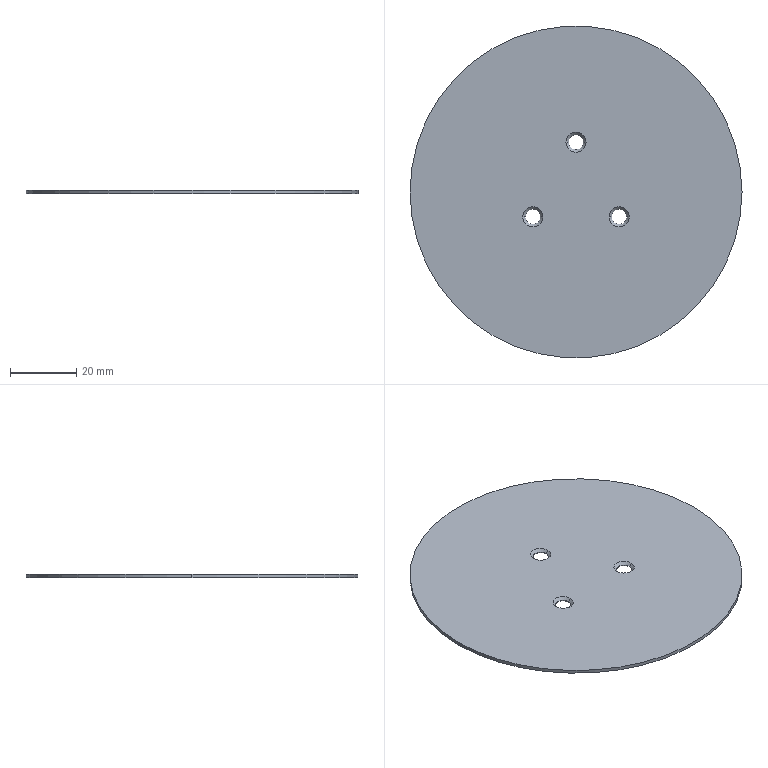Part | SolidWorks | features Chamfer 1, Extrusion 1 | 1 solid | 16 faces | box 100 x 100 x 1 mm | volume 7791 mm3 | cylinder 8 | cone 6 | plane 2 | commonest cylinder face diameters 4.5 x6 100 x2
STEP:
#1=CARTESIAN_POINT('',(-2.25,15.,0.2));
#2=VERTEX_POINT('',#1);
#3=CARTESIAN_POINT('',(2.25,15.,0.2));
#4=VERTEX_POINT('',#3);
#5=CARTESIAN_POINT('',(0.,15.,0.2));
#6=DIRECTION('',(0.,0.,1.));
#7=DIRECTION('',(1.,0.,0.));
#8=AXIS2_PLACEMENT_3D('',#5,#6,#7);
#9=CIRCLE('',#8,2.25);
#10=EDGE_CURVE('',#2,#4,#9,.T.);
#11=ORIENTED_EDGE('',*,*,#10,.F.);
#12=CARTESIAN_POINT('',(-3.05,15.,1.));
#13=VERTEX_POINT('',#12);
#14=CARTESIAN_POINT('',(-2.25,15.,0.2));
#15=DIRECTION('',(-0.7071,0.,0.7071));
#16=VECTOR('',#15,1000.);
#17=LINE('',#14,#16);
#18=EDGE_CURVE('',#2,#13,#17,.T.);
#19=ORIENTED_EDGE('',*,*,#18,.T.);
#20=CARTESIAN_POINT('',(3.05,15.,1.));
#21=VERTEX_POINT('',#20);
#22=CARTESIAN_POINT('',(0.,15.,1.));
#23=DIRECTION('',(0.,0.,-1.));
#24=DIRECTION('',(1.,0.,0.));
#25=AXIS2_PLACEMENT_3D('',#22,#23,#24);
#26=CIRCLE('',#25,3.05);
#27=EDGE_CURVE('',#21,#13,#26,.T.);
#28=ORIENTED_EDGE('',*,*,#27,.F.);
#29=CARTESIAN_POINT('',(2.25,15.,0.2));
#30=DIRECTION('',(0.7071,0.,0.7071));
#31=VECTOR('',#30,1000.);
#32=LINE('',#29,#31);
#33=EDGE_CURVE('',#4,#21,#32,.T.);
#34=ORIENTED_EDGE('',*,*,#33,.F.);
#35=EDGE_LOOP('',(#11,#19,#28,#34));
#36=FACE_OUTER_BOUND('',#35,.T.);
#37=CARTESIAN_POINT('',(0.,15.,0.2));
#38=DIRECTION('',(0.,0.,1.));
#39=DIRECTION('',(1.,0.,0.));
#40=AXIS2_PLACEMENT_3D('',#37,#38,#39);
#41=CONICAL_SURFACE('',#40,2.25,0.7854);
#42=ADVANCED_FACE('',(#36),#41,.F.);
#43=CARTESIAN_POINT('',(-15.24,-7.5,0.2));
#44=VERTEX_POINT('',#43);
#45=CARTESIAN_POINT('',(-10.74,-7.5,0.2));
#46=VERTEX_POINT('',#45);
#47=CARTESIAN_POINT('',(-12.99,-7.5,0.2));
#48=DIRECTION('',(0.,0.,1.));
#49=DIRECTION('',(1.,0.,0.));
#50=AXIS2_PLACEMENT_3D('',#47,#48,#49);
#51=CIRCLE('',#50,2.25);
#52=EDGE_CURVE('',#44,#46,#51,.T.);
#53=ORIENTED_EDGE('',*,*,#52,.F.);
#54=CARTESIAN_POINT('',(-16.04,-7.5,1.));
#55=VERTEX_POINT('',#54);
#56=CARTESIAN_POINT('',(-15.24,-7.5,0.2));
#57=DIRECTION('',(-0.7071,0.,0.7071));
#58=VECTOR('',#57,1000.);
#59=LINE('',#56,#58);
#60=EDGE_CURVE('',#44,#55,#59,.T.);
#61=ORIENTED_EDGE('',*,*,#60,.T.);
#62=CARTESIAN_POINT('',(-9.94,-7.5,1.));
#63=VERTEX_POINT('',#62);
#64=CARTESIAN_POINT('',(-12.99,-7.5,1.));
#65=DIRECTION('',(0.,0.,-1.));
#66=DIRECTION('',(1.,0.,0.));
#67=AXIS2_PLACEMENT_3D('',#64,#65,#66);
#68=CIRCLE('',#67,3.05);
#69=EDGE_CURVE('',#63,#55,#68,.T.);
#70=ORIENTED_EDGE('',*,*,#69,.F.);
#71=CARTESIAN_POINT('',(-10.74,-7.5,0.2));
#72=DIRECTION('',(0.7071,0.,0.7071));
#73=VECTOR('',#72,1000.);
#74=LINE('',#71,#73);
#75=EDGE_CURVE('',#46,#63,#74,.T.);
#76=ORIENTED_EDGE('',*,*,#75,.F.);
#77=EDGE_LOOP('',(#53,#61,#70,#76));
#78=FACE_OUTER_BOUND('',#77,.T.);
#79=CARTESIAN_POINT('',(-12.99,-7.5,0.2));
#80=DIRECTION('',(0.,0.,1.));
#81=DIRECTION('',(1.,0.,0.));
#82=AXIS2_PLACEMENT_3D('',#79,#80,#81);
#83=CONICAL_SURFACE('',#82,2.25,0.7854);
#84=ADVANCED_FACE('',(#78),#83,.F.);
#85=CARTESIAN_POINT('',(10.74,-7.5,0.2));
#86=VERTEX_POINT('',#85);
#87=CARTESIAN_POINT('',(15.24,-7.5,0.2));
#88=VERTEX_POINT('',#87);
#89=CARTESIAN_POINT('',(12.99,-7.5,0.2));
#90=DIRECTION('',(0.,0.,1.));
#91=DIRECTION('',(1.,0.,0.));
#92=AXIS2_PLACEMENT_3D('',#89,#90,#91);
#93=CIRCLE('',#92,2.25);
#94=EDGE_CURVE('',#86,#88,#93,.T.);
#95=ORIENTED_EDGE('',*,*,#94,.F.);
#96=CARTESIAN_POINT('',(9.94,-7.5,1.));
#97=VERTEX_POINT('',#96);
#98=CARTESIAN_POINT('',(10.74,-7.5,0.2));
#99=DIRECTION('',(-0.7071,0.,0.7071));
#100=VECTOR('',#99,1000.);
#101=LINE('',#98,#100);
#102=EDGE_CURVE('',#86,#97,#101,.T.);
#103=ORIENTED_EDGE('',*,*,#102,.T.);
#104=CARTESIAN_POINT('',(16.04,-7.5,1.));
#105=VERTEX_POINT('',#104);
#106=CARTESIAN_POINT('',(12.99,-7.5,1.));
#107=DIRECTION('',(0.,0.,-1.));
#108=DIRECTION('',(1.,0.,0.));
#109=AXIS2_PLACEMENT_3D('',#106,#107,#108);
#110=CIRCLE('',#109,3.05);
#111=EDGE_CURVE('',#105,#97,#110,.T.);
#112=ORIENTED_EDGE('',*,*,#111,.F.);
#113=CARTESIAN_POINT('',(15.24,-7.5,0.2));
#114=DIRECTION('',(0.7071,0.,0.7071));
#115=VECTOR('',#114,1000.);
#116=LINE('',#113,#115);
#117=EDGE_CURVE('',#88,#105,#116,.T.);
#118=ORIENTED_EDGE('',*,*,#117,.F.);
#119=EDGE_LOOP('',(#95,#103,#112,#118));
#120=FACE_OUTER_BOUND('',#119,.T.);
#121=CARTESIAN_POINT('',(12.99,-7.5,0.2));
#122=DIRECTION('',(0.,0.,1.));
#123=DIRECTION('',(1.,0.,0.));
#124=AXIS2_PLACEMENT_3D('',#121,#122,#123);
#125=CONICAL_SURFACE('',#124,2.25,0.7854);
#126=ADVANCED_FACE('',(#120),#125,.F.);
#127=ORIENTED_EDGE('',*,*,#52,.T.);
#128=CARTESIAN_POINT('',(-10.74,-7.5,0.));
#129=VERTEX_POINT('',#128);
#130=CARTESIAN_POINT('',(-10.74,-7.5,1.));
#131=DIRECTION('',(0.,0.,-1.));
#132=VECTOR('',#131,1000.);
#133=LINE('',#130,#132);
#134=EDGE_CURVE('',#46,#129,#133,.T.);
#135=ORIENTED_EDGE('',*,*,#134,.T.);
#136=CARTESIAN_POINT('',(-15.24,-7.5,0.));
#137=VERTEX_POINT('',#136);
#138=CARTESIAN_POINT('',(-12.99,-7.5,0.));
#139=DIRECTION('',(0.,0.,1.));
#140=DIRECTION('',(1.,0.,0.));
#141=AXIS2_PLACEMENT_3D('',#138,#139,#140);
#142=CIRCLE('',#141,2.25);
#143=EDGE_CURVE('',#137,#129,#142,.T.);
#144=ORIENTED_EDGE('',*,*,#143,.F.);
#145=CARTESIAN_POINT('',(-15.24,-7.5,1.));
#146=DIRECTION('',(0.,0.,-1.));
#147=VECTOR('',#146,1000.);
#148=LINE('',#145,#147);
#149=EDGE_CURVE('',#44,#137,#148,.T.);
#150=ORIENTED_EDGE('',*,*,#149,.F.);
#151=EDGE_LOOP('',(#127,#135,#144,#150));
#152=FACE_OUTER_BOUND('',#151,.T.);
#153=CARTESIAN_POINT('',(-12.99,-7.5,1.));
#154=DIRECTION('',(0.,0.,-1.));
#155=DIRECTION('',(-1.,0.,0.));
#156=AXIS2_PLACEMENT_3D('',#153,#154,#155);
#157=CYLINDRICAL_SURFACE('',#156,2.25);
#158=ADVANCED_FACE('',(#152),#157,.F.);
#159=ORIENTED_EDGE('',*,*,#94,.T.);
#160=CARTESIAN_POINT('',(15.24,-7.5,0.));
#161=VERTEX_POINT('',#160);
#162=CARTESIAN_POINT('',(15.24,-7.5,1.));
#163=DIRECTION('',(0.,0.,-1.));
#164=VECTOR('',#163,1000.);
#165=LINE('',#162,#164);
#166=EDGE_CURVE('',#88,#161,#165,.T.);
#167=ORIENTED_EDGE('',*,*,#166,.T.);
#168=CARTESIAN_POINT('',(10.74,-7.5,0.));
#169=VERTEX_POINT('',#168);
#170=CARTESIAN_POINT('',(12.99,-7.5,0.));
#171=DIRECTION('',(0.,0.,1.));
#172=DIRECTION('',(1.,0.,0.));
#173=AXIS2_PLACEMENT_3D('',#170,#171,#172);
#174=CIRCLE('',#173,2.25);
#175=EDGE_CURVE('',#169,#161,#174,.T.);
#176=ORIENTED_EDGE('',*,*,#175,.F.);
#177=CARTESIAN_POINT('',(10.74,-7.5,1.));
#178=DIRECTION('',(0.,0.,-1.));
#179=VECTOR('',#178,1000.);
#180=LINE('',#177,#179);
#181=EDGE_CURVE('',#86,#169,#180,.T.);
#182=ORIENTED_EDGE('',*,*,#181,.F.);
#183=EDGE_LOOP('',(#159,#167,#176,#182));
#184=FACE_OUTER_BOUND('',#183,.T.);
#185=CARTESIAN_POINT('',(12.99,-7.5,1.));
#186=DIRECTION('',(0.,0.,-1.));
#187=DIRECTION('',(-1.,0.,0.));
#188=AXIS2_PLACEMENT_3D('',#185,#186,#187);
#189=CYLINDRICAL_SURFACE('',#188,2.25);
#190=ADVANCED_FACE('',(#184),#189,.F.);
#191=ORIENTED_EDGE('',*,*,#10,.T.);
#192=CARTESIAN_POINT('',(2.25,15.,0.));
#193=VERTEX_POINT('',#192);
#194=CARTESIAN_POINT('',(2.25,15.,1.));
#195=DIRECTION('',(0.,0.,-1.));
#196=VECTOR('',#195,1000.);
#197=LINE('',#194,#196);
#198=EDGE_CURVE('',#4,#193,#197,.T.);
#199=ORIENTED_EDGE('',*,*,#198,.T.);
#200=CARTESIAN_POINT('',(-2.25,15.,0.));
#201=VERTEX_POINT('',#200);
#202=CARTESIAN_POINT('',(0.,15.,0.));
#203=DIRECTION('',(0.,0.,1.));
#204=DIRECTION('',(1.,0.,0.));
#205=AXIS2_PLACEMENT_3D('',#202,#203,#204);
#206=CIRCLE('',#205,2.25);
#207=EDGE_CURVE('',#201,#193,#206,.T.);
#208=ORIENTED_EDGE('',*,*,#207,.F.);
#209=CARTESIAN_POINT('',(-2.25,15.,1.));
#210=DIRECTION('',(0.,0.,-1.));
#211=VECTOR('',#210,1000.);
#212=LINE('',#209,#211);
#213=EDGE_CURVE('',#2,#201,#212,.T.);
#214=ORIENTED_EDGE('',*,*,#213,.F.);
#215=EDGE_LOOP('',(#191,#199,#208,#214));
#216=FACE_OUTER_BOUND('',#215,.T.);
#217=CARTESIAN_POINT('',(0.,15.,1.));
#218=DIRECTION('',(0.,0.,-1.));
#219=DIRECTION('',(-1.,0.,0.));
#220=AXIS2_PLACEMENT_3D('',#217,#218,#219);
#221=CYLINDRICAL_SURFACE('',#220,2.25);
#222=ADVANCED_FACE('',(#216),#221,.F.);
#223=CARTESIAN_POINT('',(50.,0.,1.));
#224=VERTEX_POINT('',#223);
#225=CARTESIAN_POINT('',(-50.,0.,1.));
#226=VERTEX_POINT('',#225);
#227=CARTESIAN_POINT('',(0.,0.,1.));
#228=DIRECTION('',(0.,0.,1.));
#229=DIRECTION('',(1.,0.,0.));
#230=AXIS2_PLACEMENT_3D('',#227,#228,#229);
#231=CIRCLE('',#230,50.);
#232=EDGE_CURVE('',#224,#226,#231,.T.);
#233=ORIENTED_EDGE('',*,*,#232,.F.);
#234=CARTESIAN_POINT('',(50.,0.,0.));
#235=VERTEX_POINT('',#234);
#236=CARTESIAN_POINT('',(50.,0.,1.));
#237=DIRECTION('',(0.,0.,-1.));
#238=VECTOR('',#237,1000.);
#239=LINE('',#236,#238);
#240=EDGE_CURVE('',#224,#235,#239,.T.);
#241=ORIENTED_EDGE('',*,*,#240,.T.);
#242=CARTESIAN_POINT('',(-50.,0.,0.));
#243=VERTEX_POINT('',#242);
#244=CARTESIAN_POINT('',(0.,0.,0.));
#245=DIRECTION('',(0.,0.,1.));
#246=DIRECTION('',(1.,0.,0.));
#247=AXIS2_PLACEMENT_3D('',#244,#245,#246);
#248=CIRCLE('',#247,50.);
#249=EDGE_CURVE('',#235,#243,#248,.T.);
#250=ORIENTED_EDGE('',*,*,#249,.T.);
#251=CARTESIAN_POINT('',(-50.,0.,1.));
#252=DIRECTION('',(0.,0.,-1.));
#253=VECTOR('',#252,1000.);
#254=LINE('',#251,#253);
#255=EDGE_CURVE('',#226,#243,#254,.T.);
#256=ORIENTED_EDGE('',*,*,#255,.F.);
#257=EDGE_LOOP('',(#233,#241,#250,#256));
#258=FACE_OUTER_BOUND('',#257,.T.);
#259=CARTESIAN_POINT('',(0.,0.,1.));
#260=DIRECTION('',(0.,0.,-1.));
#261=DIRECTION('',(-1.,0.,0.));
#262=AXIS2_PLACEMENT_3D('',#259,#260,#261);
#263=CYLINDRICAL_SURFACE('',#262,50.);
#264=ADVANCED_FACE('',(#258),#263,.T.);
#265=ORIENTED_EDGE('',*,*,#111,.T.);
#266=CARTESIAN_POINT('',(12.99,-7.5,1.));
#267=DIRECTION('',(0.,0.,-1.));
#268=DIRECTION('',(1.,0.,0.));
#269=AXIS2_PLACEMENT_3D('',#266,#267,#268);
#270=CIRCLE('',#269,3.05);
#271=EDGE_CURVE('',#97,#105,#270,.T.);
#272=ORIENTED_EDGE('',*,*,#271,.T.);
#273=EDGE_LOOP('',(#265,#272));
#274=FACE_BOUND('',#273,.T.);
#275=ORIENTED_EDGE('',*,*,#69,.T.);
#276=CARTESIAN_POINT('',(-12.99,-7.5,1.));
#277=DIRECTION('',(0.,0.,-1.));
#278=DIRECTION('',(1.,0.,0.));
#279=AXIS2_PLACEMENT_3D('',#276,#277,#278);
#280=CIRCLE('',#279,3.05);
#281=EDGE_CURVE('',#55,#63,#280,.T.);
#282=ORIENTED_EDGE('',*,*,#281,.T.);
#283=EDGE_LOOP('',(#275,#282));
#284=FACE_BOUND('',#283,.T.);
#285=ORIENTED_EDGE('',*,*,#27,.T.);
#286=CARTESIAN_POINT('',(0.,15.,1.));
#287=DIRECTION('',(0.,0.,-1.));
#288=DIRECTION('',(1.,0.,0.));
#289=AXIS2_PLACEMENT_3D('',#286,#287,#288);
#290=CIRCLE('',#289,3.05);
#291=EDGE_CURVE('',#13,#21,#290,.T.);
#292=ORIENTED_EDGE('',*,*,#291,.T.);
#293=EDGE_LOOP('',(#285,#292));
#294=FACE_BOUND('',#293,.T.);
#295=CARTESIAN_POINT('',(0.,0.,1.));
#296=DIRECTION('',(0.,0.,1.));
#297=DIRECTION('',(1.,0.,0.));
#298=AXIS2_PLACEMENT_3D('',#295,#296,#297);
#299=CIRCLE('',#298,50.);
#300=EDGE_CURVE('',#226,#224,#299,.T.);
#301=ORIENTED_EDGE('',*,*,#300,.T.);
#302=ORIENTED_EDGE('',*,*,#232,.T.);
#303=EDGE_LOOP('',(#301,#302));
#304=FACE_OUTER_BOUND('',#303,.T.);
#305=CARTESIAN_POINT('',(0.,0.,1.));
#306=DIRECTION('',(0.,0.,1.));
#307=DIRECTION('',(1.,0.,0.));
#308=AXIS2_PLACEMENT_3D('',#305,#306,#307);
#309=PLANE('',#308);
#310=ADVANCED_FACE('',(#274,#284,#294,#304),#309,.T.);
#311=ORIENTED_EDGE('',*,*,#175,.T.);
#312=CARTESIAN_POINT('',(12.99,-7.5,0.));
#313=DIRECTION('',(0.,0.,1.));
#314=DIRECTION('',(1.,0.,0.));
#315=AXIS2_PLACEMENT_3D('',#312,#313,#314);
#316=CIRCLE('',#315,2.25);
#317=EDGE_CURVE('',#161,#169,#316,.T.);
#318=ORIENTED_EDGE('',*,*,#317,.T.);
#319=EDGE_LOOP('',(#311,#318));
#320=FACE_BOUND('',#319,.T.);
#321=CARTESIAN_POINT('',(0.,0.,0.));
#322=DIRECTION('',(0.,0.,1.));
#323=DIRECTION('',(1.,0.,0.));
#324=AXIS2_PLACEMENT_3D('',#321,#322,#323);
#325=CIRCLE('',#324,50.);
#326=EDGE_CURVE('',#243,#235,#325,.T.);
#327=ORIENTED_EDGE('',*,*,#326,.F.);
#328=ORIENTED_EDGE('',*,*,#249,.F.);
#329=EDGE_LOOP('',(#327,#328));
#330=FACE_OUTER_BOUND('',#329,.T.);
#331=ORIENTED_EDGE('',*,*,#207,.T.);
#332=CARTESIAN_POINT('',(0.,15.,0.));
#333=DIRECTION('',(0.,0.,1.));
#334=DIRECTION('',(1.,0.,0.));
#335=AXIS2_PLACEMENT_3D('',#332,#333,#334);
#336=CIRCLE('',#335,2.25);
#337=EDGE_CURVE('',#193,#201,#336,.T.);
#338=ORIENTED_EDGE('',*,*,#337,.T.);
#339=EDGE_LOOP('',(#331,#338));
#340=FACE_BOUND('',#339,.T.);
#341=ORIENTED_EDGE('',*,*,#143,.T.);
#342=CARTESIAN_POINT('',(-12.99,-7.5,0.));
#343=DIRECTION('',(0.,0.,1.));
#344=DIRECTION('',(1.,0.,0.));
#345=AXIS2_PLACEMENT_3D('',#342,#343,#344);
#346=CIRCLE('',#345,2.25);
#347=EDGE_CURVE('',#129,#137,#346,.T.);
#348=ORIENTED_EDGE('',*,*,#347,.T.);
#349=EDGE_LOOP('',(#341,#348));
#350=FACE_BOUND('',#349,.T.);
#351=CARTESIAN_POINT('',(0.,0.,0.));
#352=DIRECTION('',(0.,0.,1.));
#353=DIRECTION('',(1.,0.,0.));
#354=AXIS2_PLACEMENT_3D('',#351,#352,#353);
#355=PLANE('',#354);
#356=ADVANCED_FACE('',(#320,#330,#340,#350),#355,.F.);
#357=ORIENTED_EDGE('',*,*,#240,.F.);
#358=ORIENTED_EDGE('',*,*,#300,.F.);
#359=ORIENTED_EDGE('',*,*,#255,.T.);
#360=ORIENTED_EDGE('',*,*,#326,.T.);
#361=EDGE_LOOP('',(#357,#358,#359,#360));
#362=FACE_OUTER_BOUND('',#361,.T.);
#363=CARTESIAN_POINT('',(0.,0.,1.));
#364=DIRECTION('',(0.,0.,-1.));
#365=DIRECTION('',(-1.,0.,0.));
#366=AXIS2_PLACEMENT_3D('',#363,#364,#365);
#367=CYLINDRICAL_SURFACE('',#366,50.);
#368=ADVANCED_FACE('',(#362),#367,.T.);
#369=ORIENTED_EDGE('',*,*,#198,.F.);
#370=CARTESIAN_POINT('',(0.,15.,0.2));
#371=DIRECTION('',(0.,0.,1.));
#372=DIRECTION('',(1.,0.,0.));
#373=AXIS2_PLACEMENT_3D('',#370,#371,#372);
#374=CIRCLE('',#373,2.25);
#375=EDGE_CURVE('',#4,#2,#374,.T.);
#376=ORIENTED_EDGE('',*,*,#375,.T.);
#377=ORIENTED_EDGE('',*,*,#213,.T.);
#378=ORIENTED_EDGE('',*,*,#337,.F.);
#379=EDGE_LOOP('',(#369,#376,#377,#378));
#380=FACE_OUTER_BOUND('',#379,.T.);
#381=CARTESIAN_POINT('',(0.,15.,1.));
#382=DIRECTION('',(0.,0.,-1.));
#383=DIRECTION('',(-1.,0.,0.));
#384=AXIS2_PLACEMENT_3D('',#381,#382,#383);
#385=CYLINDRICAL_SURFACE('',#384,2.25);
#386=ADVANCED_FACE('',(#380),#385,.F.);
#387=ORIENTED_EDGE('',*,*,#166,.F.);
#388=CARTESIAN_POINT('',(12.99,-7.5,0.2));
#389=DIRECTION('',(0.,0.,1.));
#390=DIRECTION('',(1.,0.,0.));
#391=AXIS2_PLACEMENT_3D('',#388,#389,#390);
#392=CIRCLE('',#391,2.25);
#393=EDGE_CURVE('',#88,#86,#392,.T.);
#394=ORIENTED_EDGE('',*,*,#393,.T.);
#395=ORIENTED_EDGE('',*,*,#181,.T.);
#396=ORIENTED_EDGE('',*,*,#317,.F.);
#397=EDGE_LOOP('',(#387,#394,#395,#396));
#398=FACE_OUTER_BOUND('',#397,.T.);
#399=CARTESIAN_POINT('',(12.99,-7.5,1.));
#400=DIRECTION('',(0.,0.,-1.));
#401=DIRECTION('',(-1.,0.,0.));
#402=AXIS2_PLACEMENT_3D('',#399,#400,#401);
#403=CYLINDRICAL_SURFACE('',#402,2.25);
#404=ADVANCED_FACE('',(#398),#403,.F.);
#405=ORIENTED_EDGE('',*,*,#134,.F.);
#406=CARTESIAN_POINT('',(-12.99,-7.5,0.2));
#407=DIRECTION('',(0.,0.,1.));
#408=DIRECTION('',(1.,0.,0.));
#409=AXIS2_PLACEMENT_3D('',#406,#407,#408);
#410=CIRCLE('',#409,2.25);
#411=EDGE_CURVE('',#46,#44,#410,.T.);
#412=ORIENTED_EDGE('',*,*,#411,.T.);
#413=ORIENTED_EDGE('',*,*,#149,.T.);
#414=ORIENTED_EDGE('',*,*,#347,.F.);
#415=EDGE_LOOP('',(#405,#412,#413,#414));
#416=FACE_OUTER_BOUND('',#415,.T.);
#417=CARTESIAN_POINT('',(-12.99,-7.5,1.));
#418=DIRECTION('',(0.,0.,-1.));
#419=DIRECTION('',(-1.,0.,0.));
#420=AXIS2_PLACEMENT_3D('',#417,#418,#419);
#421=CYLINDRICAL_SURFACE('',#420,2.25);
#422=ADVANCED_FACE('',(#416),#421,.F.);
#423=ORIENTED_EDGE('',*,*,#102,.F.);
#424=ORIENTED_EDGE('',*,*,#393,.F.);
#425=ORIENTED_EDGE('',*,*,#117,.T.);
#426=ORIENTED_EDGE('',*,*,#271,.F.);
#427=EDGE_LOOP('',(#423,#424,#425,#426));
#428=FACE_OUTER_BOUND('',#427,.T.);
#429=CARTESIAN_POINT('',(12.99,-7.5,0.2));
#430=DIRECTION('',(0.,0.,1.));
#431=DIRECTION('',(1.,0.,0.));
#432=AXIS2_PLACEMENT_3D('',#429,#430,#431);
#433=CONICAL_SURFACE('',#432,2.25,0.7854);
#434=ADVANCED_FACE('',(#428),#433,.F.);
#435=ORIENTED_EDGE('',*,*,#60,.F.);
#436=ORIENTED_EDGE('',*,*,#411,.F.);
#437=ORIENTED_EDGE('',*,*,#75,.T.);
#438=ORIENTED_EDGE('',*,*,#281,.F.);
#439=EDGE_LOOP('',(#435,#436,#437,#438));
#440=FACE_OUTER_BOUND('',#439,.T.);
#441=CARTESIAN_POINT('',(-12.99,-7.5,0.2));
#442=DIRECTION('',(0.,0.,1.));
#443=DIRECTION('',(1.,0.,0.));
#444=AXIS2_PLACEMENT_3D('',#441,#442,#443);
#445=CONICAL_SURFACE('',#444,2.25,0.7854);
#446=ADVANCED_FACE('',(#440),#445,.F.);
#447=ORIENTED_EDGE('',*,*,#18,.F.);
#448=ORIENTED_EDGE('',*,*,#375,.F.);
#449=ORIENTED_EDGE('',*,*,#33,.T.);
#450=ORIENTED_EDGE('',*,*,#291,.F.);
#451=EDGE_LOOP('',(#447,#448,#449,#450));
#452=FACE_OUTER_BOUND('',#451,.T.);
#453=CARTESIAN_POINT('',(0.,15.,0.2));
#454=DIRECTION('',(0.,0.,1.));
#455=DIRECTION('',(1.,0.,0.));
#456=AXIS2_PLACEMENT_3D('',#453,#454,#455);
#457=CONICAL_SURFACE('',#456,2.25,0.7854);
#458=ADVANCED_FACE('',(#452),#457,.F.);
#459=CLOSED_SHELL('',(#42,#84,#126,#158,#190,#222,#264,#310,#356,#368,#386,#404,#422,#434,#446,#458));
#460=MANIFOLD_SOLID_BREP('',#459);
#461=CARTESIAN_POINT('',(0.,0.,0.));
#462=DIRECTION('',(0.,0.,1.));
#463=DIRECTION('',(1.,0.,0.));
#464=AXIS2_PLACEMENT_3D('',#461,#462,#463);
#465=(LENGTH_UNIT()NAMED_UNIT(*)SI_UNIT(.MILLI.,.METRE.));
#466=UNCERTAINTY_MEASURE_WITH_UNIT(LENGTH_MEASURE(0.00001),#465,'','');
#467=(NAMED_UNIT(*)PLANE_ANGLE_UNIT()SI_UNIT($,.RADIAN.));
#468=(NAMED_UNIT(*)SI_UNIT($,.STERADIAN.)SOLID_ANGLE_UNIT());
#469=(GEOMETRIC_REPRESENTATION_CONTEXT(3)GLOBAL_UNCERTAINTY_ASSIGNED_CONTEXT((#466))GLOBAL_UNIT_ASSIGNED_CONTEXT((#465,#467,#468))REPRESENTATION_CONTEXT('',''));
#470=ADVANCED_BREP_SHAPE_REPRESENTATION('',(#460,#464),#469);